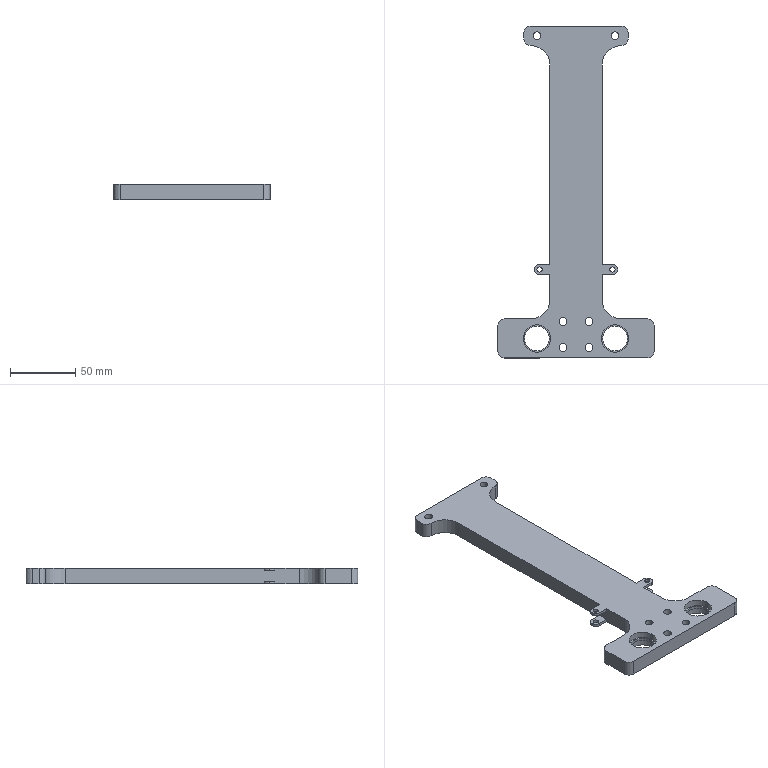Part | SolidWorks | features ICE 8, Fillet 2, Cut 1, Extrusion 1 | 1 solid | 78 faces | box 120 x 255 x 12 mm | volume 150718 mm3 | cylinder 50 | plane 28 | commonest cylinder face diameters 6 x12 4 x8 10 x8 21 x8 8 x6 19 x4